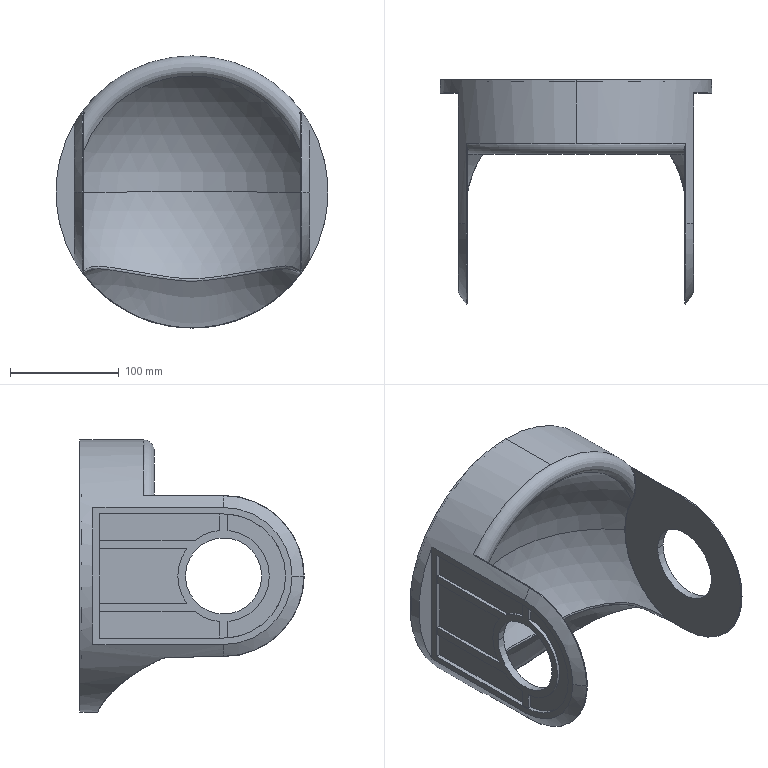Part | SolidWorks | features Fillet 16, Cut 11, ICE 3, MirrorPattern 2, PlanarSurface 2, CirPattern 1, NetBlend 1, RevCut 1, Revolution 1, SewRefSurface 1, SurfCut 1 | 1 solid | 187 faces | box 250 x 205.985 x 250 mm | volume 931758 mm3 | cylinder 63 | plane 57 | spline 33 | torus 24 | sphere 10 | commonest cylinder face diameters 5 x16 84 x10 6 x8 1 x6 2 x5 70 x4